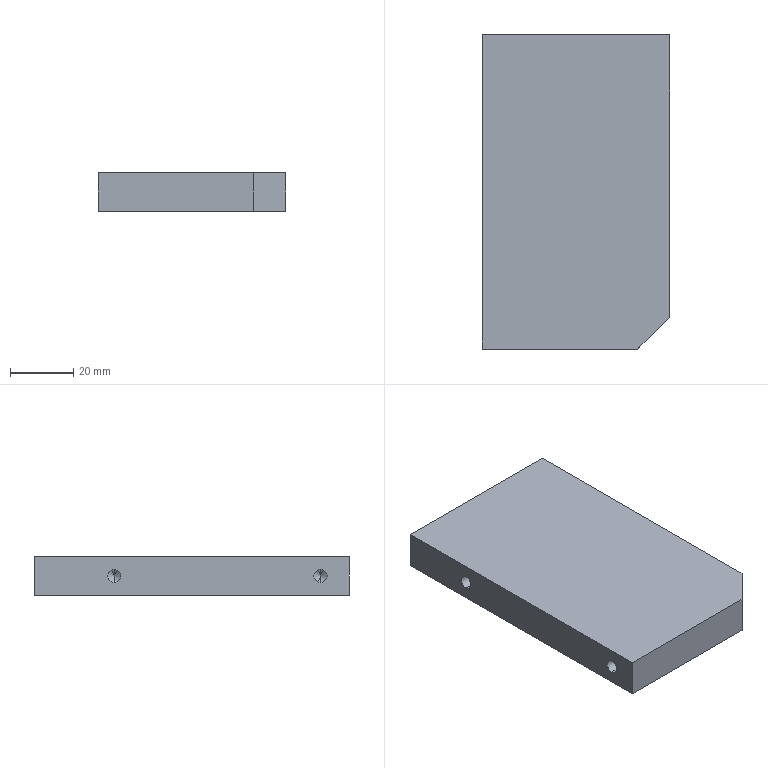Part | STEP file | 0245_202_Rib | 1 solid | 23 faces | box 59 x 99 x 12 mm | volume 68782 mm3 | cylinder 8 | cone 8 | plane 7 | commonest cylinder face diameters 4.2 x8
STEP:
#1=CARTESIAN_POINT('',(0.,0.,0.));
#2=DIRECTION('',(0.,0.,1.));
#3=DIRECTION('',(1.,0.,0.));
#4=AXIS2_PLACEMENT_3D('',#1,#2,#3);
#5=CARTESIAN_POINT('',(50.,-12.4,-3.9));
#6=VERTEX_POINT('',#5);
#7=CARTESIAN_POINT('',(50.,0.,-3.9));
#8=VERTEX_POINT('',#7);
#9=CARTESIAN_POINT('',(50.,0.,-3.9));
#10=DIRECTION('',(0.,1.,0.));
#11=VECTOR('',#10,1.);
#12=LINE('',#9,#11);
#13=CARTESIAN_POINT('',(50.,0.,-6.));
#14=DIRECTION('',(0.,1.,0.));
#15=DIRECTION('',(0.,0.,1.));
#16=AXIS2_PLACEMENT_3D('',#13,#14,#15);
#17=CYLINDRICAL_SURFACE('',#16,2.1);
#18=CARTESIAN_POINT('',(6.283,0.));
#19=DIRECTION('',(0.,1.));
#20=VECTOR('',#19,1.);
#21=LINE('',#18,#20);
#22=(GEOMETRIC_REPRESENTATION_CONTEXT(2)PARAMETRIC_REPRESENTATION_CONTEXT()REPRESENTATION_CONTEXT('',''));
#23=DEFINITIONAL_REPRESENTATION('',(#21),#22);
#24=PCURVE('',#17,#23);
#25=CARTESIAN_POINT('',(50.,0.,-6.));
#26=DIRECTION('',(0.,1.,0.));
#27=DIRECTION('',(0.,0.,1.));
#28=AXIS2_PLACEMENT_3D('',#25,#26,#27);
#29=CYLINDRICAL_SURFACE('',#28,2.1);
#30=CARTESIAN_POINT('',(0.,0.));
#31=DIRECTION('',(0.,1.));
#32=VECTOR('',#31,1.);
#33=LINE('',#30,#32);
#34=(GEOMETRIC_REPRESENTATION_CONTEXT(2)PARAMETRIC_REPRESENTATION_CONTEXT()REPRESENTATION_CONTEXT('',''));
#35=DEFINITIONAL_REPRESENTATION('',(#33),#34);
#36=PCURVE('',#29,#35);
#37=SURFACE_CURVE('',#12,(#24,#36),.PCURVE_S1.);
#38=EDGE_CURVE('',#6,#8,#37,.T.);
#39=ORIENTED_EDGE('',*,*,#38,.T.);
#40=CARTESIAN_POINT('',(50.,0.,-8.1));
#41=VERTEX_POINT('',#40);
#42=CARTESIAN_POINT('',(50.,0.,-6.));
#43=DIRECTION('',(0.,1.,0.));
#44=DIRECTION('',(0.,0.,1.));
#45=AXIS2_PLACEMENT_3D('',#42,#43,#44);
#46=CIRCLE('',#45,2.1);
#47=CARTESIAN_POINT('',(0.,0.));
#48=DIRECTION('',(1.,0.));
#49=VECTOR('',#48,1.);
#50=LINE('',#47,#49);
#51=(GEOMETRIC_REPRESENTATION_CONTEXT(2)PARAMETRIC_REPRESENTATION_CONTEXT()REPRESENTATION_CONTEXT('',''));
#52=DEFINITIONAL_REPRESENTATION('',(#50),#51);
#53=PCURVE('',#17,#52);
#54=CARTESIAN_POINT('',(0.,0.,-12.));
#55=DIRECTION('',(0.,1.,0.));
#56=DIRECTION('',(0.,0.,1.));
#57=AXIS2_PLACEMENT_3D('',#54,#55,#56);
#58=PLANE('',#57);
#59=CARTESIAN_POINT('',(6.,50.));
#60=DIRECTION('',(1.,0.));
#61=AXIS2_PLACEMENT_2D('',#59,#60);
#62=CIRCLE('',#61,2.1);
#63=(GEOMETRIC_REPRESENTATION_CONTEXT(2)PARAMETRIC_REPRESENTATION_CONTEXT()REPRESENTATION_CONTEXT('',''));
#64=DEFINITIONAL_REPRESENTATION('',(#62),#63);
#65=PCURVE('',#58,#64);
#66=SURFACE_CURVE('',#46,(#53,#65),.PCURVE_S1.);
#67=EDGE_CURVE('',#41,#8,#66,.T.);
#68=ORIENTED_EDGE('',*,*,#67,.F.);
#69=CARTESIAN_POINT('',(50.,-12.4,-8.1));
#70=VERTEX_POINT('',#69);
#71=CARTESIAN_POINT('',(50.,0.,-8.1));
#72=DIRECTION('',(0.,1.,0.));
#73=VECTOR('',#72,1.);
#74=LINE('',#71,#73);
#75=CARTESIAN_POINT('',(3.142,0.));
#76=DIRECTION('',(0.,1.));
#77=VECTOR('',#76,1.);
#78=LINE('',#75,#77);
#79=(GEOMETRIC_REPRESENTATION_CONTEXT(2)PARAMETRIC_REPRESENTATION_CONTEXT()REPRESENTATION_CONTEXT('',''));
#80=DEFINITIONAL_REPRESENTATION('',(#78),#79);
#81=PCURVE('',#17,#80);
#82=CARTESIAN_POINT('',(3.142,0.));
#83=DIRECTION('',(0.,1.));
#84=VECTOR('',#83,1.);
#85=LINE('',#82,#84);
#86=(GEOMETRIC_REPRESENTATION_CONTEXT(2)PARAMETRIC_REPRESENTATION_CONTEXT()REPRESENTATION_CONTEXT('',''));
#87=DEFINITIONAL_REPRESENTATION('',(#85),#86);
#88=PCURVE('',#29,#87);
#89=SURFACE_CURVE('',#74,(#81,#88),.PCURVE_S1.);
#90=EDGE_CURVE('',#70,#41,#89,.T.);
#91=ORIENTED_EDGE('',*,*,#90,.F.);
#92=CARTESIAN_POINT('',(50.,-12.4,-6.));
#93=DIRECTION('',(0.,1.,0.));
#94=DIRECTION('',(0.,0.,1.));
#95=AXIS2_PLACEMENT_3D('',#92,#93,#94);
#96=CIRCLE('',#95,2.1);
#97=CARTESIAN_POINT('',(0.,-12.4));
#98=DIRECTION('',(1.,0.));
#99=VECTOR('',#98,1.);
#100=LINE('',#97,#99);
#101=(GEOMETRIC_REPRESENTATION_CONTEXT(2)PARAMETRIC_REPRESENTATION_CONTEXT()REPRESENTATION_CONTEXT('',''));
#102=DEFINITIONAL_REPRESENTATION('',(#100),#101);
#103=PCURVE('',#17,#102);
#104=CARTESIAN_POINT('',(50.,-12.4,-6.));
#105=DIRECTION('',(0.,1.,0.));
#106=DIRECTION('',(0.,0.,1.));
#107=AXIS2_PLACEMENT_3D('',#104,#105,#106);
#108=CONICAL_SURFACE('',#107,2.1,1.03);
#109=CARTESIAN_POINT('',(0.,0.));
#110=DIRECTION('',(1.,0.));
#111=VECTOR('',#110,1.);
#112=LINE('',#109,#111);
#113=(GEOMETRIC_REPRESENTATION_CONTEXT(2)PARAMETRIC_REPRESENTATION_CONTEXT()REPRESENTATION_CONTEXT('',''));
#114=DEFINITIONAL_REPRESENTATION('',(#112),#113);
#115=PCURVE('',#108,#114);
#116=SURFACE_CURVE('',#96,(#103,#115),.PCURVE_S1.);
#117=EDGE_CURVE('',#70,#6,#116,.T.);
#118=ORIENTED_EDGE('',*,*,#117,.T.);
#119=EDGE_LOOP('',(#39,#68,#91,#118));
#120=FACE_BOUND('',#119,.F.);
#121=ADVANCED_FACE('',(#120),#17,.F.);
#122=ORIENTED_EDGE('',*,*,#117,.F.);
#123=CARTESIAN_POINT('',(50.,-13.662,-6.));
#124=VERTEX_POINT('',#123);
#125=CARTESIAN_POINT('',(50.,-12.4,-8.1));
#126=DIRECTION('',(0.,0.515,-0.8572));
#127=VECTOR('',#126,1.);
#128=LINE('',#125,#127);
#129=CARTESIAN_POINT('',(3.142,-1.262));
#130=CARTESIAN_POINT('',(3.142,-1.243));
#131=CARTESIAN_POINT('',(3.142,-1.204));
#132=CARTESIAN_POINT('',(3.142,-1.147));
#133=CARTESIAN_POINT('',(3.142,-1.09));
#134=CARTESIAN_POINT('',(3.142,-1.032));
#135=CARTESIAN_POINT('',(3.142,-0.975));
#136=CARTESIAN_POINT('',(3.142,-0.9177));
#137=CARTESIAN_POINT('',(3.142,-0.8603));
#138=CARTESIAN_POINT('',(3.142,-0.803));
#139=CARTESIAN_POINT('',(3.142,-0.7456));
#140=CARTESIAN_POINT('',(3.142,-0.6883));
#141=CARTESIAN_POINT('',(3.142,-0.6309));
#142=CARTESIAN_POINT('',(3.142,-0.5735));
#143=CARTESIAN_POINT('',(3.142,-0.5162));
#144=CARTESIAN_POINT('',(3.142,-0.4588));
#145=CARTESIAN_POINT('',(3.142,-0.4015));
#146=CARTESIAN_POINT('',(3.142,-0.3441));
#147=CARTESIAN_POINT('',(3.142,-0.2868));
#148=CARTESIAN_POINT('',(3.142,-0.2294));
#149=CARTESIAN_POINT('',(3.142,-0.1721));
#150=CARTESIAN_POINT('',(3.142,-0.1147));
#151=CARTESIAN_POINT('',(3.142,-0.05735));
#152=CARTESIAN_POINT('',(3.142,-0.01912));
#153=CARTESIAN_POINT('',(3.142,0.));
#154=B_SPLINE_CURVE_WITH_KNOTS('',3,(#129,#130,#131,#132,#133,#134,#135,#136,#137,#138,#139,#140,#141,#142,#143,#144,#145,#146,#147,#148,#149,#150,#151,#152,#153),.UNSPECIFIED.,.F.,.F.,(4,1,1,1,1,1,1,1,1,1,1,1,1,1,1,1,1,1,1,1,1,1,4),(-2.45,-2.339,-2.227,-2.116,-2.004,-1.893,-1.782,-1.67,-1.559,-1.448,-1.336,-1.225,-1.114,-1.002,-0.8909,-0.7795,-0.6682,-0.5568,-0.4454,-0.3341,-0.2227,-0.1114,0.),.UNSPECIFIED.);
#155=(GEOMETRIC_REPRESENTATION_CONTEXT(2)PARAMETRIC_REPRESENTATION_CONTEXT()REPRESENTATION_CONTEXT('',''));
#156=DEFINITIONAL_REPRESENTATION('',(#154),#155);
#157=PCURVE('',#108,#156);
#158=CARTESIAN_POINT('',(50.,-12.4,-6.));
#159=DIRECTION('',(0.,1.,0.));
#160=DIRECTION('',(0.,0.,1.));
#161=AXIS2_PLACEMENT_3D('',#158,#159,#160);
#162=CONICAL_SURFACE('',#161,2.1,1.03);
#163=CARTESIAN_POINT('',(3.142,-1.262));
#164=CARTESIAN_POINT('',(3.142,-1.243));
#165=CARTESIAN_POINT('',(3.142,-1.204));
#166=CARTESIAN_POINT('',(3.142,-1.147));
#167=CARTESIAN_POINT('',(3.142,-1.09));
#168=CARTESIAN_POINT('',(3.142,-1.032));
#169=CARTESIAN_POINT('',(3.142,-0.975));
#170=CARTESIAN_POINT('',(3.142,-0.9177));
#171=CARTESIAN_POINT('',(3.142,-0.8603));
#172=CARTESIAN_POINT('',(3.142,-0.803));
#173=CARTESIAN_POINT('',(3.142,-0.7456));
#174=CARTESIAN_POINT('',(3.142,-0.6883));
#175=CARTESIAN_POINT('',(3.142,-0.6309));
#176=CARTESIAN_POINT('',(3.142,-0.5735));
#177=CARTESIAN_POINT('',(3.142,-0.5162));
#178=CARTESIAN_POINT('',(3.142,-0.4588));
#179=CARTESIAN_POINT('',(3.142,-0.4015));
#180=CARTESIAN_POINT('',(3.142,-0.3441));
#181=CARTESIAN_POINT('',(3.142,-0.2868));
#182=CARTESIAN_POINT('',(3.142,-0.2294));
#183=CARTESIAN_POINT('',(3.142,-0.1721));
#184=CARTESIAN_POINT('',(3.142,-0.1147));
#185=CARTESIAN_POINT('',(3.142,-0.05735));
#186=CARTESIAN_POINT('',(3.142,-0.01912));
#187=CARTESIAN_POINT('',(3.142,0.));
#188=B_SPLINE_CURVE_WITH_KNOTS('',3,(#163,#164,#165,#166,#167,#168,#169,#170,#171,#172,#173,#174,#175,#176,#177,#178,#179,#180,#181,#182,#183,#184,#185,#186,#187),.UNSPECIFIED.,.F.,.F.,(4,1,1,1,1,1,1,1,1,1,1,1,1,1,1,1,1,1,1,1,1,1,4),(-2.45,-2.339,-2.227,-2.116,-2.004,-1.893,-1.782,-1.67,-1.559,-1.448,-1.336,-1.225,-1.114,-1.002,-0.8909,-0.7795,-0.6682,-0.5568,-0.4454,-0.3341,-0.2227,-0.1114,0.),.UNSPECIFIED.);
#189=(GEOMETRIC_REPRESENTATION_CONTEXT(2)PARAMETRIC_REPRESENTATION_CONTEXT()REPRESENTATION_CONTEXT('',''));
#190=DEFINITIONAL_REPRESENTATION('',(#188),#189);
#191=PCURVE('',#162,#190);
#192=SURFACE_CURVE('',#128,(#157,#191),.PCURVE_S1.);
#193=EDGE_CURVE('',#124,#70,#192,.T.);
#194=ORIENTED_EDGE('',*,*,#193,.F.);
#195=CARTESIAN_POINT('',(50.,-12.4,-3.9));
#196=DIRECTION('',(0.,0.515,0.8572));
#197=VECTOR('',#196,1.);
#198=LINE('',#195,#197);
#199=CARTESIAN_POINT('',(6.283,0.));
#200=DIRECTION('',(0.,1.));
#201=VECTOR('',#200,1.);
#202=LINE('',#199,#201);
#203=(GEOMETRIC_REPRESENTATION_CONTEXT(2)PARAMETRIC_REPRESENTATION_CONTEXT()REPRESENTATION_CONTEXT('',''));
#204=DEFINITIONAL_REPRESENTATION('',(#202),#203);
#205=PCURVE('',#108,#204);
#206=CARTESIAN_POINT('',(0.,0.));
#207=DIRECTION('',(0.,1.));
#208=VECTOR('',#207,1.);
#209=LINE('',#206,#208);
#210=(GEOMETRIC_REPRESENTATION_CONTEXT(2)PARAMETRIC_REPRESENTATION_CONTEXT()REPRESENTATION_CONTEXT('',''));
#211=DEFINITIONAL_REPRESENTATION('',(#209),#210);
#212=PCURVE('',#162,#211);
#213=SURFACE_CURVE('',#198,(#205,#212),.PCURVE_S1.);
#214=EDGE_CURVE('',#124,#6,#213,.T.);
#215=ORIENTED_EDGE('',*,*,#214,.T.);
#216=EDGE_LOOP('',(#122,#194,#215));
#217=FACE_BOUND('',#216,.F.);
#218=ADVANCED_FACE('',(#217),#108,.F.);
#219=CARTESIAN_POINT('',(20.,-12.4,-3.9));
#220=VERTEX_POINT('',#219);
#221=CARTESIAN_POINT('',(20.,0.,-3.9));
#222=VERTEX_POINT('',#221);
#223=CARTESIAN_POINT('',(20.,0.,-3.9));
#224=DIRECTION('',(0.,1.,0.));
#225=VECTOR('',#224,1.);
#226=LINE('',#223,#225);
#227=CARTESIAN_POINT('',(20.,0.,-6.));
#228=DIRECTION('',(0.,1.,0.));
#229=DIRECTION('',(0.,0.,1.));
#230=AXIS2_PLACEMENT_3D('',#227,#228,#229);
#231=CYLINDRICAL_SURFACE('',#230,2.1);
#232=CARTESIAN_POINT('',(6.283,0.));
#233=DIRECTION('',(0.,1.));
#234=VECTOR('',#233,1.);
#235=LINE('',#232,#234);
#236=(GEOMETRIC_REPRESENTATION_CONTEXT(2)PARAMETRIC_REPRESENTATION_CONTEXT()REPRESENTATION_CONTEXT('',''));
#237=DEFINITIONAL_REPRESENTATION('',(#235),#236);
#238=PCURVE('',#231,#237);
#239=CARTESIAN_POINT('',(20.,0.,-6.));
#240=DIRECTION('',(0.,1.,0.));
#241=DIRECTION('',(0.,0.,1.));
#242=AXIS2_PLACEMENT_3D('',#239,#240,#241);
#243=CYLINDRICAL_SURFACE('',#242,2.1);
#244=CARTESIAN_POINT('',(0.,0.));
#245=DIRECTION('',(0.,1.));
#246=VECTOR('',#245,1.);
#247=LINE('',#244,#246);
#248=(GEOMETRIC_REPRESENTATION_CONTEXT(2)PARAMETRIC_REPRESENTATION_CONTEXT()REPRESENTATION_CONTEXT('',''));
#249=DEFINITIONAL_REPRESENTATION('',(#247),#248);
#250=PCURVE('',#243,#249);
#251=SURFACE_CURVE('',#226,(#238,#250),.PCURVE_S1.);
#252=EDGE_CURVE('',#220,#222,#251,.T.);
#253=ORIENTED_EDGE('',*,*,#252,.T.);
#254=CARTESIAN_POINT('',(20.,0.,-8.1));
#255=VERTEX_POINT('',#254);
#256=CARTESIAN_POINT('',(20.,0.,-6.));
#257=DIRECTION('',(0.,1.,0.));
#258=DIRECTION('',(0.,0.,1.));
#259=AXIS2_PLACEMENT_3D('',#256,#257,#258);
#260=CIRCLE('',#259,2.1);
#261=CARTESIAN_POINT('',(0.,0.));
#262=DIRECTION('',(1.,0.));
#263=VECTOR('',#262,1.);
#264=LINE('',#261,#263);
#265=(GEOMETRIC_REPRESENTATION_CONTEXT(2)PARAMETRIC_REPRESENTATION_CONTEXT()REPRESENTATION_CONTEXT('',''));
#266=DEFINITIONAL_REPRESENTATION('',(#264),#265);
#267=PCURVE('',#231,#266);
#268=CARTESIAN_POINT('',(6.,20.));
#269=DIRECTION('',(1.,0.));
#270=AXIS2_PLACEMENT_2D('',#268,#269);
#271=CIRCLE('',#270,2.1);
#272=(GEOMETRIC_REPRESENTATION_CONTEXT(2)PARAMETRIC_REPRESENTATION_CONTEXT()REPRESENTATION_CONTEXT('',''));
#273=DEFINITIONAL_REPRESENTATION('',(#271),#272);
#274=PCURVE('',#58,#273);
#275=SURFACE_CURVE('',#260,(#267,#274),.PCURVE_S1.);
#276=EDGE_CURVE('',#255,#222,#275,.T.);
#277=ORIENTED_EDGE('',*,*,#276,.F.);
#278=CARTESIAN_POINT('',(20.,-12.4,-8.1));
#279=VERTEX_POINT('',#278);
#280=CARTESIAN_POINT('',(20.,0.,-8.1));
#281=DIRECTION('',(0.,1.,0.));
#282=VECTOR('',#281,1.);
#283=LINE('',#280,#282);
#284=CARTESIAN_POINT('',(3.142,0.));
#285=DIRECTION('',(0.,1.));
#286=VECTOR('',#285,1.);
#287=LINE('',#284,#286);
#288=(GEOMETRIC_REPRESENTATION_CONTEXT(2)PARAMETRIC_REPRESENTATION_CONTEXT()REPRESENTATION_CONTEXT('',''));
#289=DEFINITIONAL_REPRESENTATION('',(#287),#288);
#290=PCURVE('',#231,#289);
#291=CARTESIAN_POINT('',(3.142,0.));
#292=DIRECTION('',(0.,1.));
#293=VECTOR('',#292,1.);
#294=LINE('',#291,#293);
#295=(GEOMETRIC_REPRESENTATION_CONTEXT(2)PARAMETRIC_REPRESENTATION_CONTEXT()REPRESENTATION_CONTEXT('',''));
#296=DEFINITIONAL_REPRESENTATION('',(#294),#295);
#297=PCURVE('',#243,#296);
#298=SURFACE_CURVE('',#283,(#290,#297),.PCURVE_S1.);
#299=EDGE_CURVE('',#279,#255,#298,.T.);
#300=ORIENTED_EDGE('',*,*,#299,.F.);
#301=CARTESIAN_POINT('',(20.,-12.4,-6.));
#302=DIRECTION('',(0.,1.,0.));
#303=DIRECTION('',(0.,0.,1.));
#304=AXIS2_PLACEMENT_3D('',#301,#302,#303);
#305=CIRCLE('',#304,2.1);
#306=CARTESIAN_POINT('',(0.,-12.4));
#307=DIRECTION('',(1.,0.));
#308=VECTOR('',#307,1.);
#309=LINE('',#306,#308);
#310=(GEOMETRIC_REPRESENTATION_CONTEXT(2)PARAMETRIC_REPRESENTATION_CONTEXT()REPRESENTATION_CONTEXT('',''));
#311=DEFINITIONAL_REPRESENTATION('',(#309),#310);
#312=PCURVE('',#231,#311);
#313=CARTESIAN_POINT('',(20.,-12.4,-6.));
#314=DIRECTION('',(0.,1.,0.));
#315=DIRECTION('',(0.,0.,1.));
#316=AXIS2_PLACEMENT_3D('',#313,#314,#315);
#317=CONICAL_SURFACE('',#316,2.1,1.03);
#318=CARTESIAN_POINT('',(0.,0.));
#319=DIRECTION('',(1.,0.));
#320=VECTOR('',#319,1.);
#321=LINE('',#318,#320);
#322=(GEOMETRIC_REPRESENTATION_CONTEXT(2)PARAMETRIC_REPRESENTATION_CONTEXT()REPRESENTATION_CONTEXT('',''));
#323=DEFINITIONAL_REPRESENTATION('',(#321),#322);
#324=PCURVE('',#317,#323);
#325=SURFACE_CURVE('',#305,(#312,#324),.PCURVE_S1.);
#326=EDGE_CURVE('',#279,#220,#325,.T.);
#327=ORIENTED_EDGE('',*,*,#326,.T.);
#328=EDGE_LOOP('',(#253,#277,#300,#327));
#329=FACE_BOUND('',#328,.F.);
#330=ADVANCED_FACE('',(#329),#231,.F.);
#331=ORIENTED_EDGE('',*,*,#326,.F.);
#332=CARTESIAN_POINT('',(20.,-13.662,-6.));
#333=VERTEX_POINT('',#332);
#334=CARTESIAN_POINT('',(20.,-12.4,-8.1));
#335=DIRECTION('',(0.,0.515,-0.8572));
#336=VECTOR('',#335,1.);
#337=LINE('',#334,#336);
#338=CARTESIAN_POINT('',(3.142,0.));
#339=DIRECTION('',(0.,1.));
#340=VECTOR('',#339,1.);
#341=LINE('',#338,#340);
#342=(GEOMETRIC_REPRESENTATION_CONTEXT(2)PARAMETRIC_REPRESENTATION_CONTEXT()REPRESENTATION_CONTEXT('',''));
#343=DEFINITIONAL_REPRESENTATION('',(#341),#342);
#344=PCURVE('',#317,#343);
#345=CARTESIAN_POINT('',(20.,-12.4,-6.));
#346=DIRECTION('',(0.,1.,0.));
#347=DIRECTION('',(0.,0.,1.));
#348=AXIS2_PLACEMENT_3D('',#345,#346,#347);
#349=CONICAL_SURFACE('',#348,2.1,1.03);
#350=CARTESIAN_POINT('',(3.142,0.));
#351=DIRECTION('',(0.,1.));
#352=VECTOR('',#351,1.);
#353=LINE('',#350,#352);
#354=(GEOMETRIC_REPRESENTATION_CONTEXT(2)PARAMETRIC_REPRESENTATION_CONTEXT()REPRESENTATION_CONTEXT('',''));
#355=DEFINITIONAL_REPRESENTATION('',(#353),#354);
#356=PCURVE('',#349,#355);
#357=SURFACE_CURVE('',#337,(#344,#356),.PCURVE_S1.);
#358=EDGE_CURVE('',#333,#279,#357,.T.);
#359=ORIENTED_EDGE('',*,*,#358,.F.);
#360=CARTESIAN_POINT('',(20.,-12.4,-3.9));
#361=DIRECTION('',(0.,0.515,0.8572));
#362=VECTOR('',#361,1.);
#363=LINE('',#360,#362);
#364=CARTESIAN_POINT('',(6.283,0.));
#365=DIRECTION('',(0.,1.));
#366=VECTOR('',#365,1.);
#367=LINE('',#364,#366);
#368=(GEOMETRIC_REPRESENTATION_CONTEXT(2)PARAMETRIC_REPRESENTATION_CONTEXT()REPRESENTATION_CONTEXT('',''));
#369=DEFINITIONAL_REPRESENTATION('',(#367),#368);
#370=PCURVE('',#317,#369);
#371=CARTESIAN_POINT('',(0.,0.));
#372=DIRECTION('',(0.,1.));
#373=VECTOR('',#372,1.);
#374=LINE('',#371,#373);
#375=(GEOMETRIC_REPRESENTATION_CONTEXT(2)PARAMETRIC_REPRESENTATION_CONTEXT()REPRESENTATION_CONTEXT('',''));
#376=DEFINITIONAL_REPRESENTATION('',(#374),#375);
#377=PCURVE('',#349,#376);
#378=SURFACE_CURVE('',#363,(#370,#377),.PCURVE_S1.);
#379=EDGE_CURVE('',#333,#220,#378,.T.);
#380=ORIENTED_EDGE('',*,*,#379,.T.);
#381=EDGE_LOOP('',(#331,#359,#380));
#382=FACE_BOUND('',#381,.F.);
#383=ADVANCED_FACE('',(#382),#317,.F.);
#384=CARTESIAN_POINT('',(12.4,-25.,-3.9));
#385=VERTEX_POINT('',#384);
#386=CARTESIAN_POINT('',(0.,-25.,-3.9));
#387=VERTEX_POINT('',#386);
#388=CARTESIAN_POINT('',(0.,-25.,-3.9));
#389=DIRECTION('',(-1.,0.,0.));
#390=VECTOR('',#389,1.);
#391=LINE('',#388,#390);
#392=CARTESIAN_POINT('',(0.,-25.,-6.));
#393=DIRECTION('',(-1.,0.,0.));
#394=DIRECTION('',(0.,0.,1.));
#395=AXIS2_PLACEMENT_3D('',#392,#393,#394);
#396=CYLINDRICAL_SURFACE('',#395,2.1);
#397=CARTESIAN_POINT('',(6.283,0.));
#398=DIRECTION('',(0.,1.));
#399=VECTOR('',#398,1.);
#400=LINE('',#397,#399);
#401=(GEOMETRIC_REPRESENTATION_CONTEXT(2)PARAMETRIC_REPRESENTATION_CONTEXT()REPRESENTATION_CONTEXT('',''));
#402=DEFINITIONAL_REPRESENTATION('',(#400),#401);
#403=PCURVE('',#396,#402);
#404=CARTESIAN_POINT('',(0.,-25.,-6.));
#405=DIRECTION('',(-1.,0.,0.));
#406=DIRECTION('',(0.,0.,1.));
#407=AXIS2_PLACEMENT_3D('',#404,#405,#406);
#408=CYLINDRICAL_SURFACE('',#407,2.1);
#409=CARTESIAN_POINT('',(0.,0.));
#410=DIRECTION('',(0.,1.));
#411=VECTOR('',#410,1.);
#412=LINE('',#409,#411);
#413=(GEOMETRIC_REPRESENTATION_CONTEXT(2)PARAMETRIC_REPRESENTATION_CONTEXT()REPRESENTATION_CONTEXT('',''));
#414=DEFINITIONAL_REPRESENTATION('',(#412),#413);
#415=PCURVE('',#408,#414);
#416=SURFACE_CURVE('',#391,(#403,#415),.PCURVE_S1.);
#417=EDGE_CURVE('',#385,#387,#416,.T.);
#418=ORIENTED_EDGE('',*,*,#417,.T.);
#419=CARTESIAN_POINT('',(0.,-25.,-8.1));
#420=VERTEX_POINT('',#419);
#421=CARTESIAN_POINT('',(0.,-25.,-6.));
#422=DIRECTION('',(-1.,0.,0.));
#423=DIRECTION('',(0.,0.,1.));
#424=AXIS2_PLACEMENT_3D('',#421,#422,#423);
#425=CIRCLE('',#424,2.1);
#426=CARTESIAN_POINT('',(0.,0.));
#427=DIRECTION('',(1.,0.));
#428=VECTOR('',#427,1.);
#429=LINE('',#426,#428);
#430=(GEOMETRIC_REPRESENTATION_CONTEXT(2)PARAMETRIC_REPRESENTATION_CONTEXT()REPRESENTATION_CONTEXT('',''));
#431=DEFINITIONAL_REPRESENTATION('',(#429),#430);
#432=PCURVE('',#396,#431);
#433=CARTESIAN_POINT('',(0.,-99.,-12.));
#434=DIRECTION('',(-1.,0.,0.));
#435=DIRECTION('',(0.,0.,1.));
#436=AXIS2_PLACEMENT_3D('',#433,#434,#435);
#437=PLANE('',#436);
#438=CARTESIAN_POINT('',(6.,74.));
#439=DIRECTION('',(1.,0.));
#440=AXIS2_PLACEMENT_2D('',#438,#439);
#441=CIRCLE('',#440,2.1);
#442=(GEOMETRIC_REPRESENTATION_CONTEXT(2)PARAMETRIC_REPRESENTATION_CONTEXT()REPRESENTATION_CONTEXT('',''));
#443=DEFINITIONAL_REPRESENTATION('',(#441),#442);
#444=PCURVE('',#437,#443);
#445=SURFACE_CURVE('',#425,(#432,#444),.PCURVE_S1.);
#446=EDGE_CURVE('',#420,#387,#445,.T.);
#447=ORIENTED_EDGE('',*,*,#446,.F.);
#448=CARTESIAN_POINT('',(12.4,-25.,-8.1));
#449=VERTEX_POINT('',#448);
#450=CARTESIAN_POINT('',(0.,-25.,-8.1));
#451=DIRECTION('',(-1.,0.,0.));
#452=VECTOR('',#451,1.);
#453=LINE('',#450,#452);
#454=CARTESIAN_POINT('',(3.142,0.));
#455=DIRECTION('',(0.,1.));
#456=VECTOR('',#455,1.);
#457=LINE('',#454,#456);
#458=(GEOMETRIC_REPRESENTATION_CONTEXT(2)PARAMETRIC_REPRESENTATION_CONTEXT()REPRESENTATION_CONTEXT('',''));
#459=DEFINITIONAL_REPRESENTATION('',(#457),#458);
#460=PCURVE('',#396,#459);
#461=CARTESIAN_POINT('',(3.142,0.));
#462=DIRECTION('',(0.,1.));
#463=VECTOR('',#462,1.);
#464=LINE('',#461,#463);
#465=(GEOMETRIC_REPRESENTATION_CONTEXT(2)PARAMETRIC_REPRESENTATION_CONTEXT()REPRESENTATION_CONTEXT('',''));
#466=DEFINITIONAL_REPRESENTATION('',(#464),#465);
#467=PCURVE('',#408,#466);
#468=SURFACE_CURVE('',#453,(#460,#467),.PCURVE_S1.);
#469=EDGE_CURVE('',#449,#420,#468,.T.);
#470=ORIENTED_EDGE('',*,*,#469,.F.);
#471=CARTESIAN_POINT('',(12.4,-25.,-6.));
#472=DIRECTION('',(-1.,0.,0.));
#473=DIRECTION('',(0.,0.,1.));
#474=AXIS2_PLACEMENT_3D('',#471,#472,#473);
#475=CIRCLE('',#474,2.1);
#476=CARTESIAN_POINT('',(0.,-12.4));
#477=DIRECTION('',(1.,0.));
#478=VECTOR('',#477,1.);
#479=LINE('',#476,#478);
#480=(GEOMETRIC_REPRESENTATION_CONTEXT(2)PARAMETRIC_REPRESENTATION_CONTEXT()REPRESENTATION_CONTEXT('',''));
#481=DEFINITIONAL_REPRESENTATION('',(#479),#480);
#482=PCURVE('',#396,#481);
#483=CARTESIAN_POINT('',(12.4,-25.,-6.));
#484=DIRECTION('',(-1.,0.,0.));
#485=DIRECTION('',(0.,0.,1.));
#486=AXIS2_PLACEMENT_3D('',#483,#484,#485);
#487=CONICAL_SURFACE('',#486,2.1,1.03);
#488=CARTESIAN_POINT('',(0.,0.));
#489=DIRECTION('',(1.,0.));
#490=VECTOR('',#489,1.);
#491=LINE('',#488,#490);
#492=(GEOMETRIC_REPRESENTATION_CONTEXT(2)PARAMETRIC_REPRESENTATION_CONTEXT()REPRESENTATION_CONTEXT('',''));
#493=DEFINITIONAL_REPRESENTATION('',(#491),#492);
#494=PCURVE('',#487,#493);
#495=SURFACE_CURVE('',#475,(#482,#494),.PCURVE_S1.);
#496=EDGE_CURVE('',#449,#385,#495,.T.);
#497=ORIENTED_EDGE('',*,*,#496,.T.);
#498=EDGE_LOOP('',(#418,#447,#470,#497));
#499=FACE_BOUND('',#498,.F.);
#500=ADVANCED_FACE('',(#499),#396,.F.);
#501=ORIENTED_EDGE('',*,*,#496,.F.);
#502=CARTESIAN_POINT('',(13.662,-25.,-6.));
#503=VERTEX_POINT('',#502);
#504=CARTESIAN_POINT('',(12.4,-25.,-8.1));
#505=DIRECTION('',(-0.515,0.,-0.8572));
#506=VECTOR('',#505,1.);
#507=LINE('',#504,#506);
#508=CARTESIAN_POINT('',(3.142,0.));
#509=DIRECTION('',(0.,1.));
#510=VECTOR('',#509,1.);
#511=LINE('',#508,#510);
#512=(GEOMETRIC_REPRESENTATION_CONTEXT(2)PARAMETRIC_REPRESENTATION_CONTEXT()REPRESENTATION_CONTEXT('',''));
#513=DEFINITIONAL_REPRESENTATION('',(#511),#512);
#514=PCURVE('',#487,#513);
#515=CARTESIAN_POINT('',(12.4,-25.,-6.));
#516=DIRECTION('',(-1.,0.,0.));
#517=DIRECTION('',(0.,0.,1.));
#518=AXIS2_PLACEMENT_3D('',#515,#516,#517);
#519=CONICAL_SURFACE('',#518,2.1,1.03);
#520=CARTESIAN_POINT('',(3.142,0.));
#521=DIRECTION('',(0.,1.));
#522=VECTOR('',#521,1.);
#523=LINE('',#520,#522);
#524=(GEOMETRIC_REPRESENTATION_CONTEXT(2)PARAMETRIC_REPRESENTATION_CONTEXT()REPRESENTATION_CONTEXT('',''));
#525=DEFINITIONAL_REPRESENTATION('',(#523),#524);
#526=PCURVE('',#519,#525);
#527=SURFACE_CURVE('',#507,(#514,#526),.PCURVE_S1.);
#528=EDGE_CURVE('',#503,#449,#527,.T.);
#529=ORIENTED_EDGE('',*,*,#528,.F.);
#530=CARTESIAN_POINT('',(12.4,-25.,-3.9));
#531=DIRECTION('',(-0.515,0.,0.8572));
#532=VECTOR('',#531,1.);
#533=LINE('',#530,#532);
#534=CARTESIAN_POINT('',(6.283,0.));
#535=DIRECTION('',(0.,1.));
#536=VECTOR('',#535,1.);
#537=LINE('',#534,#536);
#538=(GEOMETRIC_REPRESENTATION_CONTEXT(2)PARAMETRIC_REPRESENTATION_CONTEXT()REPRESENTATION_CONTEXT('',''));
#539=DEFINITIONAL_REPRESENTATION('',(#537),#538);
#540=PCURVE('',#487,#539);
#541=CARTESIAN_POINT('',(0.,0.));
#542=DIRECTION('',(0.,1.));
#543=VECTOR('',#542,1.);
#544=LINE('',#541,#543);
#545=(GEOMETRIC_REPRESENTATION_CONTEXT(2)PARAMETRIC_REPRESENTATION_CONTEXT()REPRESENTATION_CONTEXT('',''));
#546=DEFINITIONAL_REPRESENTATION('',(#544),#545);
#547=PCURVE('',#519,#546);
#548=SURFACE_CURVE('',#533,(#540,#547),.PCURVE_S1.);
#549=EDGE_CURVE('',#503,#385,#548,.T.);
#550=ORIENTED_EDGE('',*,*,#549,.T.);
#551=EDGE_LOOP('',(#501,#529,#550));
#552=FACE_BOUND('',#551,.F.);
#553=ADVANCED_FACE('',(#552),#487,.F.);
#554=CARTESIAN_POINT('',(12.4,-90.,-3.9));
#555=VERTEX_POINT('',#554);
#556=CARTESIAN_POINT('',(0.,-90.,-3.9));
#557=VERTEX_POINT('',#556);
#558=CARTESIAN_POINT('',(0.,-90.,-3.9));
#559=DIRECTION('',(-1.,0.,0.));
#560=VECTOR('',#559,1.);
#561=LINE('',#558,#560);
#562=CARTESIAN_POINT('',(0.,-90.,-6.));
#563=DIRECTION('',(-1.,0.,0.));
#564=DIRECTION('',(0.,0.,1.));
#565=AXIS2_PLACEMENT_3D('',#562,#563,#564);
#566=CYLINDRICAL_SURFACE('',#565,2.1);
#567=CARTESIAN_POINT('',(6.283,0.));
#568=DIRECTION('',(0.,1.));
#569=VECTOR('',#568,1.);
#570=LINE('',#567,#569);
#571=(GEOMETRIC_REPRESENTATION_CONTEXT(2)PARAMETRIC_REPRESENTATION_CONTEXT()REPRESENTATION_CONTEXT('',''));
#572=DEFINITIONAL_REPRESENTATION('',(#570),#571);
#573=PCURVE('',#566,#572);
#574=CARTESIAN_POINT('',(0.,-90.,-6.));
#575=DIRECTION('',(-1.,0.,0.));
#576=DIRECTION('',(0.,0.,1.));
#577=AXIS2_PLACEMENT_3D('',#574,#575,#576);
#578=CYLINDRICAL_SURFACE('',#577,2.1);
#579=CARTESIAN_POINT('',(0.,0.));
#580=DIRECTION('',(0.,1.));
#581=VECTOR('',#580,1.);
#582=LINE('',#579,#581);
#583=(GEOMETRIC_REPRESENTATION_CONTEXT(2)PARAMETRIC_REPRESENTATION_CONTEXT()REPRESENTATION_CONTEXT('',''));
#584=DEFINITIONAL_REPRESENTATION('',(#582),#583);
#585=PCURVE('',#578,#584);
#586=SURFACE_CURVE('',#561,(#573,#585),.PCURVE_S1.);
#587=EDGE_CURVE('',#555,#557,#586,.T.);
#588=ORIENTED_EDGE('',*,*,#587,.T.);
#589=CARTESIAN_POINT('',(0.,-90.,-8.1));
#590=VERTEX_POINT('',#589);
#591=CARTESIAN_POINT('',(0.,-90.,-6.));
#592=DIRECTION('',(-1.,0.,0.));
#593=DIRECTION('',(0.,0.,1.));
#594=AXIS2_PLACEMENT_3D('',#591,#592,#593);
#595=CIRCLE('',#594,2.1);
#596=CARTESIAN_POINT('',(0.,0.));
#597=DIRECTION('',(1.,0.));
#598=VECTOR('',#597,1.);
#599=LINE('',#596,#598);
#600=(GEOMETRIC_REPRESENTATION_CONTEXT(2)PARAMETRIC_REPRESENTATION_CONTEXT()REPRESENTATION_CONTEXT('',''));
#601=DEFINITIONAL_REPRESENTATION('',(#599),#600);
#602=PCURVE('',#566,#601);
#603=CARTESIAN_POINT('',(6.,9.));
#604=DIRECTION('',(1.,0.));
#605=AXIS2_PLACEMENT_2D('',#603,#604);
#606=CIRCLE('',#605,2.1);
#607=(GEOMETRIC_REPRESENTATION_CONTEXT(2)PARAMETRIC_REPRESENTATION_CONTEXT()REPRESENTATION_CONTEXT('',''));
#608=DEFINITIONAL_REPRESENTATION('',(#606),#607);
#609=PCURVE('',#437,#608);
#610=SURFACE_CURVE('',#595,(#602,#609),.PCURVE_S1.);
#611=EDGE_CURVE('',#590,#557,#610,.T.);
#612=ORIENTED_EDGE('',*,*,#611,.F.);
#613=CARTESIAN_POINT('',(12.4,-90.,-8.1));
#614=VERTEX_POINT('',#613);
#615=CARTESIAN_POINT('',(0.,-90.,-8.1));
#616=DIRECTION('',(-1.,0.,0.));
#617=VECTOR('',#616,1.);
#618=LINE('',#615,#617);
#619=CARTESIAN_POINT('',(3.142,0.));
#620=DIRECTION('',(0.,1.));
#621=VECTOR('',#620,1.);
#622=LINE('',#619,#621);
#623=(GEOMETRIC_REPRESENTATION_CONTEXT(2)PARAMETRIC_REPRESENTATION_CONTEXT()REPRESENTATION_CONTEXT('',''));
#624=DEFINITIONAL_REPRESENTATION('',(#622),#623);
#625=PCURVE('',#566,#624);
#626=CARTESIAN_POINT('',(3.142,0.));
#627=DIRECTION('',(0.,1.));
#628=VECTOR('',#627,1.);
#629=LINE('',#626,#628);
#630=(GEOMETRIC_REPRESENTATION_CONTEXT(2)PARAMETRIC_REPRESENTATION_CONTEXT()REPRESENTATION_CONTEXT('',''));
#631=DEFINITIONAL_REPRESENTATION('',(#629),#630);
#632=PCURVE('',#578,#631);
#633=SURFACE_CURVE('',#618,(#625,#632),.PCURVE_S1.);
#634=EDGE_CURVE('',#614,#590,#633,.T.);
#635=ORIENTED_EDGE('',*,*,#634,.F.);
#636=CARTESIAN_POINT('',(12.4,-90.,-6.));
#637=DIRECTION('',(-1.,0.,0.));
#638=DIRECTION('',(0.,0.,1.));
#639=AXIS2_PLACEMENT_3D('',#636,#637,#638);
#640=CIRCLE('',#639,2.1);
#641=CARTESIAN_POINT('',(0.,-12.4));
#642=DIRECTION('',(1.,0.));
#643=VECTOR('',#642,1.);
#644=LINE('',#641,#643);
#645=(GEOMETRIC_REPRESENTATION_CONTEXT(2)PARAMETRIC_REPRESENTATION_CONTEXT()REPRESENTATION_CONTEXT('',''));
#646=DEFINITIONAL_REPRESENTATION('',(#644),#645);
#647=PCURVE('',#566,#646);
#648=CARTESIAN_POINT('',(12.4,-90.,-6.));
#649=DIRECTION('',(-1.,0.,0.));
#650=DIRECTION('',(0.,0.,1.));
#651=AXIS2_PLACEMENT_3D('',#648,#649,#650);
#652=CONICAL_SURFACE('',#651,2.1,1.03);
#653=CARTESIAN_POINT('',(0.,0.));
#654=DIRECTION('',(1.,0.));
#655=VECTOR('',#654,1.);
#656=LINE('',#653,#655);
#657=(GEOMETRIC_REPRESENTATION_CONTEXT(2)PARAMETRIC_REPRESENTATION_CONTEXT()REPRESENTATION_CONTEXT('',''));
#658=DEFINITIONAL_REPRESENTATION('',(#656),#657);
#659=PCURVE('',#652,#658);
#660=SURFACE_CURVE('',#640,(#647,#659),.PCURVE_S1.);
#661=EDGE_CURVE('',#614,#555,#660,.T.);
#662=ORIENTED_EDGE('',*,*,#661,.T.);
#663=EDGE_LOOP('',(#588,#612,#635,#662));
#664=FACE_BOUND('',#663,.F.);
#665=ADVANCED_FACE('',(#664),#566,.F.);
#666=ORIENTED_EDGE('',*,*,#661,.F.);
#667=CARTESIAN_POINT('',(13.662,-90.,-6.));
#668=VERTEX_POINT('',#667);
#669=CARTESIAN_POINT('',(12.4,-90.,-8.1));
#670=DIRECTION('',(-0.515,0.,-0.8572));
#671=VECTOR('',#670,1.);
#672=LINE('',#669,#671);
#673=CARTESIAN_POINT('',(3.142,-1.262));
#674=CARTESIAN_POINT('',(3.142,-1.243));
#675=CARTESIAN_POINT('',(3.142,-1.204));
#676=CARTESIAN_POINT('',(3.142,-1.147));
#677=CARTESIAN_POINT('',(3.142,-1.09));
#678=CARTESIAN_POINT('',(3.142,-1.032));
#679=CARTESIAN_POINT('',(3.142,-0.975));
#680=CARTESIAN_POINT('',(3.142,-0.9177));
#681=CARTESIAN_POINT('',(3.142,-0.8603));
#682=CARTESIAN_POINT('',(3.142,-0.803));
#683=CARTESIAN_POINT('',(3.142,-0.7456));
#684=CARTESIAN_POINT('',(3.142,-0.6883));
#685=CARTESIAN_POINT('',(3.142,-0.6309));
#686=CARTESIAN_POINT('',(3.142,-0.5735));
#687=CARTESIAN_POINT('',(3.142,-0.5162));
#688=CARTESIAN_POINT('',(3.142,-0.4588));
#689=CARTESIAN_POINT('',(3.142,-0.4015));
#690=CARTESIAN_POINT('',(3.142,-0.3441));
#691=CARTESIAN_POINT('',(3.142,-0.2868));
#692=CARTESIAN_POINT('',(3.142,-0.2294));
#693=CARTESIAN_POINT('',(3.142,-0.1721));
#694=CARTESIAN_POINT('',(3.142,-0.1147));
#695=CARTESIAN_POINT('',(3.142,-0.05735));
#696=CARTESIAN_POINT('',(3.142,-0.01912));
#697=CARTESIAN_POINT('',(3.142,0.));
#698=B_SPLINE_CURVE_WITH_KNOTS('',3,(#673,#674,#675,#676,#677,#678,#679,#680,#681,#682,#683,#684,#685,#686,#687,#688,#689,#690,#691,#692,#693,#694,#695,#696,#697),.UNSPECIFIED.,.F.,.F.,(4,1,1,1,1,1,1,1,1,1,1,1,1,1,1,1,1,1,1,1,1,1,4),(-2.45,-2.339,-2.227,-2.116,-2.004,-1.893,-1.782,-1.67,-1.559,-1.448,-1.336,-1.225,-1.114,-1.002,-0.8909,-0.7795,-0.6682,-0.5568,-0.4454,-0.3341,-0.2227,-0.1114,0.),.UNSPECIFIED.);
#699=(GEOMETRIC_REPRESENTATION_CONTEXT(2)PARAMETRIC_REPRESENTATION_CONTEXT()REPRESENTATION_CONTEXT('',''));
#700=DEFINITIONAL_REPRESENTATION('',(#698),#699);
#701=PCURVE('',#652,#700);
#702=CARTESIAN_POINT('',(12.4,-90.,-6.));
#703=DIRECTION('',(-1.,0.,0.));
#704=DIRECTION('',(0.,0.,1.));
#705=AXIS2_PLACEMENT_3D('',#702,#703,#704);
#706=CONICAL_SURFACE('',#705,2.1,1.03);
#707=CARTESIAN_POINT('',(3.142,-1.262));
#708=CARTESIAN_POINT('',(3.142,-1.243));
#709=CARTESIAN_POINT('',(3.142,-1.204));
#710=CARTESIAN_POINT('',(3.142,-1.147));
#711=CARTESIAN_POINT('',(3.142,-1.09));
#712=CARTESIAN_POINT('',(3.142,-1.032));
#713=CARTESIAN_POINT('',(3.142,-0.975));
#714=CARTESIAN_POINT('',(3.142,-0.9177));
#715=CARTESIAN_POINT('',(3.142,-0.8603));
#716=CARTESIAN_POINT('',(3.142,-0.803));
#717=CARTESIAN_POINT('',(3.142,-0.7456));
#718=CARTESIAN_POINT('',(3.142,-0.6883));
#719=CARTESIAN_POINT('',(3.142,-0.6309));
#720=CARTESIAN_POINT('',(3.142,-0.5735));
#721=CARTESIAN_POINT('',(3.142,-0.5162));
#722=CARTESIAN_POINT('',(3.142,-0.4588));
#723=CARTESIAN_POINT('',(3.142,-0.4015));
#724=CARTESIAN_POINT('',(3.142,-0.3441));
#725=CARTESIAN_POINT('',(3.142,-0.2868));
#726=CARTESIAN_POINT('',(3.142,-0.2294));
#727=CARTESIAN_POINT('',(3.142,-0.1721));
#728=CARTESIAN_POINT('',(3.142,-0.1147));
#729=CARTESIAN_POINT('',(3.142,-0.05735));
#730=CARTESIAN_POINT('',(3.142,-0.01912));
#731=CARTESIAN_POINT('',(3.142,0.));
#732=B_SPLINE_CURVE_WITH_KNOTS('',3,(#707,#708,#709,#710,#711,#712,#713,#714,#715,#716,#717,#718,#719,#720,#721,#722,#723,#724,#725,#726,#727,#728,#729,#730,#731),.UNSPECIFIED.,.F.,.F.,(4,1,1,1,1,1,1,1,1,1,1,1,1,1,1,1,1,1,1,1,1,1,4),(-2.45,-2.339,-2.227,-2.116,-2.004,-1.893,-1.782,-1.67,-1.559,-1.448,-1.336,-1.225,-1.114,-1.002,-0.8909,-0.7795,-0.6682,-0.5568,-0.4454,-0.3341,-0.2227,-0.1114,0.),.UNSPECIFIED.);
#733=(GEOMETRIC_REPRESENTATION_CONTEXT(2)PARAMETRIC_REPRESENTATION_CONTEXT()REPRESENTATION_CONTEXT('',''));
#734=DEFINITIONAL_REPRESENTATION('',(#732),#733);
#735=PCURVE('',#706,#734);
#736=SURFACE_CURVE('',#672,(#701,#735),.PCURVE_S1.);
#737=EDGE_CURVE('',#668,#614,#736,.T.);
#738=ORIENTED_EDGE('',*,*,#737,.F.);
#739=CARTESIAN_POINT('',(12.4,-90.,-3.9));
#740=DIRECTION('',(-0.515,0.,0.8572));
#741=VECTOR('',#740,1.);
#742=LINE('',#739,#741);
#743=CARTESIAN_POINT('',(6.283,0.));
#744=DIRECTION('',(0.,1.));
#745=VECTOR('',#744,1.);
#746=LINE('',#743,#745);
#747=(GEOMETRIC_REPRESENTATION_CONTEXT(2)PARAMETRIC_REPRESENTATION_CONTEXT()REPRESENTATION_CONTEXT('',''));
#748=DEFINITIONAL_REPRESENTATION('',(#746),#747);
#749=PCURVE('',#652,#748);
#750=CARTESIAN_POINT('',(0.,0.));
#751=DIRECTION('',(0.,1.));
#752=VECTOR('',#751,1.);
#753=LINE('',#750,#752);
#754=(GEOMETRIC_REPRESENTATION_CONTEXT(2)PARAMETRIC_REPRESENTATION_CONTEXT()REPRESENTATION_CONTEXT('',''));
#755=DEFINITIONAL_REPRESENTATION('',(#753),#754);
#756=PCURVE('',#706,#755);
#757=SURFACE_CURVE('',#742,(#749,#756),.PCURVE_S1.);
#758=EDGE_CURVE('',#668,#555,#757,.T.);
#759=ORIENTED_EDGE('',*,*,#758,.T.);
#760=EDGE_LOOP('',(#666,#738,#759));
#761=FACE_BOUND('',#760,.F.);
#762=ADVANCED_FACE('',(#761),#652,.F.);
#763=CARTESIAN_POINT('',(0.,-25.,-6.));
#764=DIRECTION('',(-1.,0.,0.));
#765=DIRECTION('',(0.,0.,1.));
#766=AXIS2_PLACEMENT_3D('',#763,#764,#765);
#767=CIRCLE('',#766,2.1);
#768=CARTESIAN_POINT('',(6.,74.));
#769=DIRECTION('',(1.,0.));
#770=AXIS2_PLACEMENT_2D('',#768,#769);
#771=CIRCLE('',#770,2.1);
#772=(GEOMETRIC_REPRESENTATION_CONTEXT(2)PARAMETRIC_REPRESENTATION_CONTEXT()REPRESENTATION_CONTEXT('',''));
#773=DEFINITIONAL_REPRESENTATION('',(#771),#772);
#774=PCURVE('',#437,#773);
#775=CARTESIAN_POINT('',(0.,0.));
#776=DIRECTION('',(1.,0.));
#777=VECTOR('',#776,1.);
#778=LINE('',#775,#777);
#779=(GEOMETRIC_REPRESENTATION_CONTEXT(2)PARAMETRIC_REPRESENTATION_CONTEXT()REPRESENTATION_CONTEXT('',''));
#780=DEFINITIONAL_REPRESENTATION('',(#778),#779);
#781=PCURVE('',#408,#780);
#782=SURFACE_CURVE('',#767,(#774,#781),.PCURVE_S1.);
#783=EDGE_CURVE('',#387,#420,#782,.T.);
#784=ORIENTED_EDGE('',*,*,#783,.F.);
#785=ORIENTED_EDGE('',*,*,#446,.F.);
#786=EDGE_LOOP('',(#784,#785));
#787=FACE_BOUND('',#786,.T.);
#788=CARTESIAN_POINT('',(0.,-90.,-6.));
#789=DIRECTION('',(-1.,0.,0.));
#790=DIRECTION('',(0.,0.,1.));
#791=AXIS2_PLACEMENT_3D('',#788,#789,#790);
#792=CIRCLE('',#791,2.1);
#793=CARTESIAN_POINT('',(6.,9.));
#794=DIRECTION('',(1.,0.));
#795=AXIS2_PLACEMENT_2D('',#793,#794);
#796=CIRCLE('',#795,2.1);
#797=(GEOMETRIC_REPRESENTATION_CONTEXT(2)PARAMETRIC_REPRESENTATION_CONTEXT()REPRESENTATION_CONTEXT('',''));
#798=DEFINITIONAL_REPRESENTATION('',(#796),#797);
#799=PCURVE('',#437,#798);
#800=CARTESIAN_POINT('',(0.,0.));
#801=DIRECTION('',(1.,0.));
#802=VECTOR('',#801,1.);
#803=LINE('',#800,#802);
#804=(GEOMETRIC_REPRESENTATION_CONTEXT(2)PARAMETRIC_REPRESENTATION_CONTEXT()REPRESENTATION_CONTEXT('',''));
#805=DEFINITIONAL_REPRESENTATION('',(#803),#804);
#806=PCURVE('',#578,#805);
#807=SURFACE_CURVE('',#792,(#799,#806),.PCURVE_S1.);
#808=EDGE_CURVE('',#557,#590,#807,.T.);
#809=ORIENTED_EDGE('',*,*,#808,.F.);
#810=ORIENTED_EDGE('',*,*,#611,.F.);
#811=EDGE_LOOP('',(#809,#810));
#812=FACE_BOUND('',#811,.T.);
#813=CARTESIAN_POINT('',(0.,0.,0.));
#814=VERTEX_POINT('',#813);
#815=CARTESIAN_POINT('',(0.,-99.,0.));
#816=VERTEX_POINT('',#815);
#817=CARTESIAN_POINT('',(0.,-99.,0.));
#818=DIRECTION('',(0.,-1.,0.));
#819=VECTOR('',#818,1.);
#820=LINE('',#817,#819);
#821=CARTESIAN_POINT('',(12.,0.));
#822=DIRECTION('',(0.,-1.));
#823=VECTOR('',#822,1.);
#824=LINE('',#821,#823);
#825=(GEOMETRIC_REPRESENTATION_CONTEXT(2)PARAMETRIC_REPRESENTATION_CONTEXT()REPRESENTATION_CONTEXT('',''));
#826=DEFINITIONAL_REPRESENTATION('',(#824),#825);
#827=PCURVE('',#437,#826);
#828=CARTESIAN_POINT('',(0.,0.,0.));
#829=DIRECTION('',(0.,0.,-1.));
#830=DIRECTION('',(-1.,0.,0.));
#831=AXIS2_PLACEMENT_3D('',#828,#829,#830);
#832=PLANE('',#831);
#833=CARTESIAN_POINT('',(0.,-99.));
#834=DIRECTION('',(0.,-1.));
#835=VECTOR('',#834,1.);
#836=LINE('',#833,#835);
#837=(GEOMETRIC_REPRESENTATION_CONTEXT(2)PARAMETRIC_REPRESENTATION_CONTEXT()REPRESENTATION_CONTEXT('',''));
#838=DEFINITIONAL_REPRESENTATION('',(#836),#837);
#839=PCURVE('',#832,#838);
#840=SURFACE_CURVE('',#820,(#827,#839),.PCURVE_S1.);
#841=EDGE_CURVE('',#814,#816,#840,.T.);
#842=ORIENTED_EDGE('',*,*,#841,.F.);
#843=CARTESIAN_POINT('',(0.,0.,-12.));
#844=VERTEX_POINT('',#843);
#845=CARTESIAN_POINT('',(0.,0.,-12.));
#846=DIRECTION('',(0.,0.,1.));
#847=VECTOR('',#846,1.);
#848=LINE('',#845,#847);
#849=CARTESIAN_POINT('',(0.,99.));
#850=DIRECTION('',(1.,0.));
#851=VECTOR('',#850,1.);
#852=LINE('',#849,#851);
#853=(GEOMETRIC_REPRESENTATION_CONTEXT(2)PARAMETRIC_REPRESENTATION_CONTEXT()REPRESENTATION_CONTEXT('',''));
#854=DEFINITIONAL_REPRESENTATION('',(#852),#853);
#855=PCURVE('',#437,#854);
#856=CARTESIAN_POINT('',(0.,0.));
#857=DIRECTION('',(1.,0.));
#858=VECTOR('',#857,1.);
#859=LINE('',#856,#858);
#860=(GEOMETRIC_REPRESENTATION_CONTEXT(2)PARAMETRIC_REPRESENTATION_CONTEXT()REPRESENTATION_CONTEXT('',''));
#861=DEFINITIONAL_REPRESENTATION('',(#859),#860);
#862=PCURVE('',#58,#861);
#863=SURFACE_CURVE('',#848,(#855,#862),.PCURVE_S1.);
#864=EDGE_CURVE('',#844,#814,#863,.T.);
#865=ORIENTED_EDGE('',*,*,#864,.F.);
#866=CARTESIAN_POINT('',(0.,-99.,-12.));
#867=VERTEX_POINT('',#866);
#868=CARTESIAN_POINT('',(0.,-99.,-12.));
#869=DIRECTION('',(0.,-1.,0.));
#870=VECTOR('',#869,1.);
#871=LINE('',#868,#870);
#872=CARTESIAN_POINT('',(0.,0.));
#873=DIRECTION('',(0.,-1.));
#874=VECTOR('',#873,1.);
#875=LINE('',#872,#874);
#876=(GEOMETRIC_REPRESENTATION_CONTEXT(2)PARAMETRIC_REPRESENTATION_CONTEXT()REPRESENTATION_CONTEXT('',''));
#877=DEFINITIONAL_REPRESENTATION('',(#875),#876);
#878=PCURVE('',#437,#877);
#879=CARTESIAN_POINT('',(0.,0.,-12.));
#880=DIRECTION('',(0.,0.,-1.));
#881=DIRECTION('',(-1.,0.,0.));
#882=AXIS2_PLACEMENT_3D('',#879,#880,#881);
#883=PLANE('',#882);
#884=CARTESIAN_POINT('',(0.,-99.));
#885=DIRECTION('',(0.,-1.));
#886=VECTOR('',#885,1.);
#887=LINE('',#884,#886);
#888=(GEOMETRIC_REPRESENTATION_CONTEXT(2)PARAMETRIC_REPRESENTATION_CONTEXT()REPRESENTATION_CONTEXT('',''));
#889=DEFINITIONAL_REPRESENTATION('',(#887),#888);
#890=PCURVE('',#883,#889);
#891=SURFACE_CURVE('',#871,(#878,#890),.PCURVE_S1.);
#892=EDGE_CURVE('',#844,#867,#891,.T.);
#893=ORIENTED_EDGE('',*,*,#892,.T.);
#894=CARTESIAN_POINT('',(0.,-99.,-12.));
#895=DIRECTION('',(0.,0.,1.));
#896=VECTOR('',#895,1.);
#897=LINE('',#894,#896);
#898=CARTESIAN_POINT('',(0.,0.));
#899=DIRECTION('',(1.,0.));
#900=VECTOR('',#899,1.);
#901=LINE('',#898,#900);
#902=(GEOMETRIC_REPRESENTATION_CONTEXT(2)PARAMETRIC_REPRESENTATION_CONTEXT()REPRESENTATION_CONTEXT('',''));
#903=DEFINITIONAL_REPRESENTATION('',(#901),#902);
#904=PCURVE('',#437,#903);
#905=CARTESIAN_POINT('',(49.,-99.,-12.));
#906=DIRECTION('',(0.,-1.,0.));
#907=DIRECTION('',(0.,0.,-1.));
#908=AXIS2_PLACEMENT_3D('',#905,#906,#907);
#909=PLANE('',#908);
#910=CARTESIAN_POINT('',(0.,-49.));
#911=DIRECTION('',(-1.,0.));
#912=VECTOR('',#911,1.);
#913=LINE('',#910,#912);
#914=(GEOMETRIC_REPRESENTATION_CONTEXT(2)PARAMETRIC_REPRESENTATION_CONTEXT()REPRESENTATION_CONTEXT('',''));
#915=DEFINITIONAL_REPRESENTATION('',(#913),#914);
#916=PCURVE('',#909,#915);
#917=SURFACE_CURVE('',#897,(#904,#916),.PCURVE_S1.);
#918=EDGE_CURVE('',#867,#816,#917,.T.);
#919=ORIENTED_EDGE('',*,*,#918,.T.);
#920=EDGE_LOOP('',(#842,#865,#893,#919));
#921=FACE_BOUND('',#920,.T.);
#922=ADVANCED_FACE('',(#787,#812,#921),#437,.T.);
#923=CARTESIAN_POINT('',(50.,0.,-6.));
#924=DIRECTION('',(0.,1.,0.));
#925=DIRECTION('',(0.,0.,1.));
#926=AXIS2_PLACEMENT_3D('',#923,#924,#925);
#927=CIRCLE('',#926,2.1);
#928=CARTESIAN_POINT('',(6.,50.));
#929=DIRECTION('',(1.,0.));
#930=AXIS2_PLACEMENT_2D('',#928,#929);
#931=CIRCLE('',#930,2.1);
#932=(GEOMETRIC_REPRESENTATION_CONTEXT(2)PARAMETRIC_REPRESENTATION_CONTEXT()REPRESENTATION_CONTEXT('',''));
#933=DEFINITIONAL_REPRESENTATION('',(#931),#932);
#934=PCURVE('',#58,#933);
#935=CARTESIAN_POINT('',(0.,0.));
#936=DIRECTION('',(1.,0.));
#937=VECTOR('',#936,1.);
#938=LINE('',#935,#937);
#939=(GEOMETRIC_REPRESENTATION_CONTEXT(2)PARAMETRIC_REPRESENTATION_CONTEXT()REPRESENTATION_CONTEXT('',''));
#940=DEFINITIONAL_REPRESENTATION('',(#938),#939);
#941=PCURVE('',#29,#940);
#942=SURFACE_CURVE('',#927,(#934,#941),.PCURVE_S1.);
#943=EDGE_CURVE('',#8,#41,#942,.T.);
#944=ORIENTED_EDGE('',*,*,#943,.F.);
#945=ORIENTED_EDGE('',*,*,#67,.F.);
#946=EDGE_LOOP('',(#944,#945));
#947=FACE_BOUND('',#946,.T.);
#948=CARTESIAN_POINT('',(20.,0.,-6.));
#949=DIRECTION('',(0.,1.,0.));
#950=DIRECTION('',(0.,0.,1.));
#951=AXIS2_PLACEMENT_3D('',#948,#949,#950);
#952=CIRCLE('',#951,2.1);
#953=CARTESIAN_POINT('',(6.,20.));
#954=DIRECTION('',(1.,0.));
#955=AXIS2_PLACEMENT_2D('',#953,#954);
#956=CIRCLE('',#955,2.1);
#957=(GEOMETRIC_REPRESENTATION_CONTEXT(2)PARAMETRIC_REPRESENTATION_CONTEXT()REPRESENTATION_CONTEXT('',''));
#958=DEFINITIONAL_REPRESENTATION('',(#956),#957);
#959=PCURVE('',#58,#958);
#960=CARTESIAN_POINT('',(0.,0.));
#961=DIRECTION('',(1.,0.));
#962=VECTOR('',#961,1.);
#963=LINE('',#960,#962);
#964=(GEOMETRIC_REPRESENTATION_CONTEXT(2)PARAMETRIC_REPRESENTATION_CONTEXT()REPRESENTATION_CONTEXT('',''));
#965=DEFINITIONAL_REPRESENTATION('',(#963),#964);
#966=PCURVE('',#243,#965);
#967=SURFACE_CURVE('',#952,(#959,#966),.PCURVE_S1.);
#968=EDGE_CURVE('',#222,#255,#967,.T.);
#969=ORIENTED_EDGE('',*,*,#968,.F.);
#970=ORIENTED_EDGE('',*,*,#276,.F.);
#971=EDGE_LOOP('',(#969,#970));
#972=FACE_BOUND('',#971,.T.);
#973=CARTESIAN_POINT('',(59.,0.,0.));
#974=VERTEX_POINT('',#973);
#975=CARTESIAN_POINT('',(0.,0.,0.));
#976=DIRECTION('',(-1.,0.,0.));
#977=VECTOR('',#976,1.);
#978=LINE('',#975,#977);
#979=CARTESIAN_POINT('',(12.,0.));
#980=DIRECTION('',(0.,-1.));
#981=VECTOR('',#980,1.);
#982=LINE('',#979,#981);
#983=(GEOMETRIC_REPRESENTATION_CONTEXT(2)PARAMETRIC_REPRESENTATION_CONTEXT()REPRESENTATION_CONTEXT('',''));
#984=DEFINITIONAL_REPRESENTATION('',(#982),#983);
#985=PCURVE('',#58,#984);
#986=CARTESIAN_POINT('',(0.,0.));
#987=DIRECTION('',(1.,0.));
#988=VECTOR('',#987,1.);
#989=LINE('',#986,#988);
#990=(GEOMETRIC_REPRESENTATION_CONTEXT(2)PARAMETRIC_REPRESENTATION_CONTEXT()REPRESENTATION_CONTEXT('',''));
#991=DEFINITIONAL_REPRESENTATION('',(#989),#990);
#992=PCURVE('',#832,#991);
#993=SURFACE_CURVE('',#978,(#985,#992),.PCURVE_S1.);
#994=EDGE_CURVE('',#974,#814,#993,.T.);
#995=ORIENTED_EDGE('',*,*,#994,.F.);
#996=CARTESIAN_POINT('',(59.,0.,-12.));
#997=VERTEX_POINT('',#996);
#998=CARTESIAN_POINT('',(59.,0.,-12.));
#999=DIRECTION('',(0.,0.,1.));
#1000=VECTOR('',#999,1.);
#1001=LINE('',#998,#1000);
#1002=CARTESIAN_POINT('',(0.,59.));
#1003=DIRECTION('',(1.,0.));
#1004=VECTOR('',#1003,1.);
#1005=LINE('',#1002,#1004);
#1006=(GEOMETRIC_REPRESENTATION_CONTEXT(2)PARAMETRIC_REPRESENTATION_CONTEXT()REPRESENTATION_CONTEXT('',''));
#1007=DEFINITIONAL_REPRESENTATION('',(#1005),#1006);
#1008=PCURVE('',#58,#1007);
#1009=CARTESIAN_POINT('',(59.,0.,-12.));
#1010=DIRECTION('',(1.,0.,0.));
#1011=DIRECTION('',(0.,1.,0.));
#1012=AXIS2_PLACEMENT_3D('',#1009,#1010,#1011);
#1013=PLANE('',#1012);
#1014=CARTESIAN_POINT('',(0.,0.));
#1015=DIRECTION('',(0.,1.));
#1016=VECTOR('',#1015,1.);
#1017=LINE('',#1014,#1016);
#1018=(GEOMETRIC_REPRESENTATION_CONTEXT(2)PARAMETRIC_REPRESENTATION_CONTEXT()REPRESENTATION_CONTEXT('',''));
#1019=DEFINITIONAL_REPRESENTATION('',(#1017),#1018);
#1020=PCURVE('',#1013,#1019);
#1021=SURFACE_CURVE('',#1001,(#1008,#1020),.PCURVE_S1.);
#1022=EDGE_CURVE('',#997,#974,#1021,.T.);
#1023=ORIENTED_EDGE('',*,*,#1022,.F.);
#1024=CARTESIAN_POINT('',(0.,0.,-12.));
#1025=DIRECTION('',(-1.,0.,0.));
#1026=VECTOR('',#1025,1.);
#1027=LINE('',#1024,#1026);
#1028=CARTESIAN_POINT('',(0.,0.));
#1029=DIRECTION('',(0.,-1.));
#1030=VECTOR('',#1029,1.);
#1031=LINE('',#1028,#1030);
#1032=(GEOMETRIC_REPRESENTATION_CONTEXT(2)PARAMETRIC_REPRESENTATION_CONTEXT()REPRESENTATION_CONTEXT('',''));
#1033=DEFINITIONAL_REPRESENTATION('',(#1031),#1032);
#1034=PCURVE('',#58,#1033);
#1035=CARTESIAN_POINT('',(0.,0.));
#1036=DIRECTION('',(1.,0.));
#1037=VECTOR('',#1036,1.);
#1038=LINE('',#1035,#1037);
#1039=(GEOMETRIC_REPRESENTATION_CONTEXT(2)PARAMETRIC_REPRESENTATION_CONTEXT()REPRESENTATION_CONTEXT('',''));
#1040=DEFINITIONAL_REPRESENTATION('',(#1038),#1039);
#1041=PCURVE('',#883,#1040);
#1042=SURFACE_CURVE('',#1027,(#1034,#1041),.PCURVE_S1.);
#1043=EDGE_CURVE('',#997,#844,#1042,.T.);
#1044=ORIENTED_EDGE('',*,*,#1043,.T.);
#1045=ORIENTED_EDGE('',*,*,#864,.T.);
#1046=EDGE_LOOP('',(#995,#1023,#1044,#1045));
#1047=FACE_BOUND('',#1046,.T.);
#1048=ADVANCED_FACE('',(#947,#972,#1047),#58,.T.);
#1049=CARTESIAN_POINT('',(59.,-89.,0.));
#1050=VERTEX_POINT('',#1049);
#1051=CARTESIAN_POINT('',(59.,0.,0.));
#1052=DIRECTION('',(0.,1.,0.));
#1053=VECTOR('',#1052,1.);
#1054=LINE('',#1051,#1053);
#1055=CARTESIAN_POINT('',(0.,12.));
#1056=DIRECTION('',(1.,0.));
#1057=VECTOR('',#1056,1.);
#1058=LINE('',#1055,#1057);
#1059=(GEOMETRIC_REPRESENTATION_CONTEXT(2)PARAMETRIC_REPRESENTATION_CONTEXT()REPRESENTATION_CONTEXT('',''));
#1060=DEFINITIONAL_REPRESENTATION('',(#1058),#1059);
#1061=PCURVE('',#1013,#1060);
#1062=CARTESIAN_POINT('',(-59.,0.));
#1063=DIRECTION('',(0.,1.));
#1064=VECTOR('',#1063,1.);
#1065=LINE('',#1062,#1064);
#1066=(GEOMETRIC_REPRESENTATION_CONTEXT(2)PARAMETRIC_REPRESENTATION_CONTEXT()REPRESENTATION_CONTEXT('',''));
#1067=DEFINITIONAL_REPRESENTATION('',(#1065),#1066);
#1068=PCURVE('',#832,#1067);
#1069=SURFACE_CURVE('',#1054,(#1061,#1068),.PCURVE_S1.);
#1070=EDGE_CURVE('',#1050,#974,#1069,.T.);
#1071=ORIENTED_EDGE('',*,*,#1070,.F.);
#1072=CARTESIAN_POINT('',(59.,-89.,-12.));
#1073=VERTEX_POINT('',#1072);
#1074=CARTESIAN_POINT('',(59.,-89.,-12.));
#1075=DIRECTION('',(0.,0.,1.));
#1076=VECTOR('',#1075,1.);
#1077=LINE('',#1074,#1076);
#1078=CARTESIAN_POINT('',(-89.,0.));
#1079=DIRECTION('',(0.,1.));
#1080=VECTOR('',#1079,1.);
#1081=LINE('',#1078,#1080);
#1082=(GEOMETRIC_REPRESENTATION_CONTEXT(2)PARAMETRIC_REPRESENTATION_CONTEXT()REPRESENTATION_CONTEXT('',''));
#1083=DEFINITIONAL_REPRESENTATION('',(#1081),#1082);
#1084=PCURVE('',#1013,#1083);
#1085=CARTESIAN_POINT('',(59.,-89.,-12.));
#1086=DIRECTION('',(0.7071,-0.7071,0.));
#1087=DIRECTION('',(0.7071,0.7071,0.));
#1088=AXIS2_PLACEMENT_3D('',#1085,#1086,#1087);
#1089=PLANE('',#1088);
#1090=CARTESIAN_POINT('',(0.,0.));
#1091=DIRECTION('',(0.,1.));
#1092=VECTOR('',#1091,1.);
#1093=LINE('',#1090,#1092);
#1094=(GEOMETRIC_REPRESENTATION_CONTEXT(2)PARAMETRIC_REPRESENTATION_CONTEXT()REPRESENTATION_CONTEXT('',''));
#1095=DEFINITIONAL_REPRESENTATION('',(#1093),#1094);
#1096=PCURVE('',#1089,#1095);
#1097=SURFACE_CURVE('',#1077,(#1084,#1096),.PCURVE_S1.);
#1098=EDGE_CURVE('',#1073,#1050,#1097,.T.);
#1099=ORIENTED_EDGE('',*,*,#1098,.F.);
#1100=CARTESIAN_POINT('',(59.,0.,-12.));
#1101=DIRECTION('',(0.,1.,0.));
#1102=VECTOR('',#1101,1.);
#1103=LINE('',#1100,#1102);
#1104=CARTESIAN_POINT('',(0.,0.));
#1105=DIRECTION('',(1.,0.));
#1106=VECTOR('',#1105,1.);
#1107=LINE('',#1104,#1106);
#1108=(GEOMETRIC_REPRESENTATION_CONTEXT(2)PARAMETRIC_REPRESENTATION_CONTEXT()REPRESENTATION_CONTEXT('',''));
#1109=DEFINITIONAL_REPRESENTATION('',(#1107),#1108);
#1110=PCURVE('',#1013,#1109);
#1111=CARTESIAN_POINT('',(-59.,0.));
#1112=DIRECTION('',(0.,1.));
#1113=VECTOR('',#1112,1.);
#1114=LINE('',#1111,#1113);
#1115=(GEOMETRIC_REPRESENTATION_CONTEXT(2)PARAMETRIC_REPRESENTATION_CONTEXT()REPRESENTATION_CONTEXT('',''));
#1116=DEFINITIONAL_REPRESENTATION('',(#1114),#1115);
#1117=PCURVE('',#883,#1116);
#1118=SURFACE_CURVE('',#1103,(#1110,#1117),.PCURVE_S1.);
#1119=EDGE_CURVE('',#1073,#997,#1118,.T.);
#1120=ORIENTED_EDGE('',*,*,#1119,.T.);
#1121=ORIENTED_EDGE('',*,*,#1022,.T.);
#1122=EDGE_LOOP('',(#1071,#1099,#1120,#1121));
#1123=FACE_BOUND('',#1122,.T.);
#1124=ADVANCED_FACE('',(#1123),#1013,.T.);
#1125=CARTESIAN_POINT('',(49.,-99.,0.));
#1126=VERTEX_POINT('',#1125);
#1127=CARTESIAN_POINT('',(59.,-89.,0.));
#1128=DIRECTION('',(0.7071,0.7071,0.));
#1129=VECTOR('',#1128,1.);
#1130=LINE('',#1127,#1129);
#1131=CARTESIAN_POINT('',(0.,12.));
#1132=DIRECTION('',(1.,0.));
#1133=VECTOR('',#1132,1.);
#1134=LINE('',#1131,#1133);
#1135=(GEOMETRIC_REPRESENTATION_CONTEXT(2)PARAMETRIC_REPRESENTATION_CONTEXT()REPRESENTATION_CONTEXT('',''));
#1136=DEFINITIONAL_REPRESENTATION('',(#1134),#1135);
#1137=PCURVE('',#1089,#1136);
#1138=CARTESIAN_POINT('',(-59.,-89.));
#1139=DIRECTION('',(-0.7071,0.7071));
#1140=VECTOR('',#1139,1.);
#1141=LINE('',#1138,#1140);
#1142=(GEOMETRIC_REPRESENTATION_CONTEXT(2)PARAMETRIC_REPRESENTATION_CONTEXT()REPRESENTATION_CONTEXT('',''));
#1143=DEFINITIONAL_REPRESENTATION('',(#1141),#1142);
#1144=PCURVE('',#832,#1143);
#1145=SURFACE_CURVE('',#1130,(#1137,#1144),.PCURVE_S1.);
#1146=EDGE_CURVE('',#1126,#1050,#1145,.T.);
#1147=ORIENTED_EDGE('',*,*,#1146,.F.);
#1148=CARTESIAN_POINT('',(49.,-99.,-12.));
#1149=VERTEX_POINT('',#1148);
#1150=CARTESIAN_POINT('',(49.,-99.,-12.));
#1151=DIRECTION('',(0.,0.,1.));
#1152=VECTOR('',#1151,1.);
#1153=LINE('',#1150,#1152);
#1154=CARTESIAN_POINT('',(-14.142,0.));
#1155=DIRECTION('',(0.,1.));
#1156=VECTOR('',#1155,1.);
#1157=LINE('',#1154,#1156);
#1158=(GEOMETRIC_REPRESENTATION_CONTEXT(2)PARAMETRIC_REPRESENTATION_CONTEXT()REPRESENTATION_CONTEXT('',''));
#1159=DEFINITIONAL_REPRESENTATION('',(#1157),#1158);
#1160=PCURVE('',#1089,#1159);
#1161=CARTESIAN_POINT('',(0.,0.));
#1162=DIRECTION('',(-1.,0.));
#1163=VECTOR('',#1162,1.);
#1164=LINE('',#1161,#1163);
#1165=(GEOMETRIC_REPRESENTATION_CONTEXT(2)PARAMETRIC_REPRESENTATION_CONTEXT()REPRESENTATION_CONTEXT('',''));
#1166=DEFINITIONAL_REPRESENTATION('',(#1164),#1165);
#1167=PCURVE('',#909,#1166);
#1168=SURFACE_CURVE('',#1153,(#1160,#1167),.PCURVE_S1.);
#1169=EDGE_CURVE('',#1149,#1126,#1168,.T.);
#1170=ORIENTED_EDGE('',*,*,#1169,.F.);
#1171=CARTESIAN_POINT('',(59.,-89.,-12.));
#1172=DIRECTION('',(0.7071,0.7071,0.));
#1173=VECTOR('',#1172,1.);
#1174=LINE('',#1171,#1173);
#1175=CARTESIAN_POINT('',(0.,0.));
#1176=DIRECTION('',(1.,0.));
#1177=VECTOR('',#1176,1.);
#1178=LINE('',#1175,#1177);
#1179=(GEOMETRIC_REPRESENTATION_CONTEXT(2)PARAMETRIC_REPRESENTATION_CONTEXT()REPRESENTATION_CONTEXT('',''));
#1180=DEFINITIONAL_REPRESENTATION('',(#1178),#1179);
#1181=PCURVE('',#1089,#1180);
#1182=CARTESIAN_POINT('',(-59.,-89.));
#1183=DIRECTION('',(-0.7071,0.7071));
#1184=VECTOR('',#1183,1.);
#1185=LINE('',#1182,#1184);
#1186=(GEOMETRIC_REPRESENTATION_CONTEXT(2)PARAMETRIC_REPRESENTATION_CONTEXT()REPRESENTATION_CONTEXT('',''));
#1187=DEFINITIONAL_REPRESENTATION('',(#1185),#1186);
#1188=PCURVE('',#883,#1187);
#1189=SURFACE_CURVE('',#1174,(#1181,#1188),.PCURVE_S1.);
#1190=EDGE_CURVE('',#1149,#1073,#1189,.T.);
#1191=ORIENTED_EDGE('',*,*,#1190,.T.);
#1192=ORIENTED_EDGE('',*,*,#1098,.T.);
#1193=EDGE_LOOP('',(#1147,#1170,#1191,#1192));
#1194=FACE_BOUND('',#1193,.T.);
#1195=ADVANCED_FACE('',(#1194),#1089,.T.);
#1196=CARTESIAN_POINT('',(49.,-99.,0.));
#1197=DIRECTION('',(1.,0.,0.));
#1198=VECTOR('',#1197,1.);
#1199=LINE('',#1196,#1198);
#1200=CARTESIAN_POINT('',(-12.,0.));
#1201=DIRECTION('',(0.,1.));
#1202=VECTOR('',#1201,1.);
#1203=LINE('',#1200,#1202);
#1204=(GEOMETRIC_REPRESENTATION_CONTEXT(2)PARAMETRIC_REPRESENTATION_CONTEXT()REPRESENTATION_CONTEXT('',''));
#1205=DEFINITIONAL_REPRESENTATION('',(#1203),#1204);
#1206=PCURVE('',#909,#1205);
#1207=CARTESIAN_POINT('',(-49.,-99.));
#1208=DIRECTION('',(-1.,0.));
#1209=VECTOR('',#1208,1.);
#1210=LINE('',#1207,#1209);
#1211=(GEOMETRIC_REPRESENTATION_CONTEXT(2)PARAMETRIC_REPRESENTATION_CONTEXT()REPRESENTATION_CONTEXT('',''));
#1212=DEFINITIONAL_REPRESENTATION('',(#1210),#1211);
#1213=PCURVE('',#832,#1212);
#1214=SURFACE_CURVE('',#1199,(#1206,#1213),.PCURVE_S1.);
#1215=EDGE_CURVE('',#816,#1126,#1214,.T.);
#1216=ORIENTED_EDGE('',*,*,#1215,.F.);
#1217=ORIENTED_EDGE('',*,*,#918,.F.);
#1218=CARTESIAN_POINT('',(49.,-99.,-12.));
#1219=DIRECTION('',(1.,0.,0.));
#1220=VECTOR('',#1219,1.);
#1221=LINE('',#1218,#1220);
#1222=CARTESIAN_POINT('',(0.,0.));
#1223=DIRECTION('',(0.,1.));
#1224=VECTOR('',#1223,1.);
#1225=LINE('',#1222,#1224);
#1226=(GEOMETRIC_REPRESENTATION_CONTEXT(2)PARAMETRIC_REPRESENTATION_CONTEXT()REPRESENTATION_CONTEXT('',''));
#1227=DEFINITIONAL_REPRESENTATION('',(#1225),#1226);
#1228=PCURVE('',#909,#1227);
#1229=CARTESIAN_POINT('',(-49.,-99.));
#1230=DIRECTION('',(-1.,0.));
#1231=VECTOR('',#1230,1.);
#1232=LINE('',#1229,#1231);
#1233=(GEOMETRIC_REPRESENTATION_CONTEXT(2)PARAMETRIC_REPRESENTATION_CONTEXT()REPRESENTATION_CONTEXT('',''));
#1234=DEFINITIONAL_REPRESENTATION('',(#1232),#1233);
#1235=PCURVE('',#883,#1234);
#1236=SURFACE_CURVE('',#1221,(#1228,#1235),.PCURVE_S1.);
#1237=EDGE_CURVE('',#867,#1149,#1236,.T.);
#1238=ORIENTED_EDGE('',*,*,#1237,.T.);
#1239=ORIENTED_EDGE('',*,*,#1169,.T.);
#1240=EDGE_LOOP('',(#1216,#1217,#1238,#1239));
#1241=FACE_BOUND('',#1240,.T.);
#1242=ADVANCED_FACE('',(#1241),#909,.T.);
#1243=ORIENTED_EDGE('',*,*,#892,.F.);
#1244=ORIENTED_EDGE('',*,*,#1043,.F.);
#1245=ORIENTED_EDGE('',*,*,#1119,.F.);
#1246=ORIENTED_EDGE('',*,*,#1190,.F.);
#1247=ORIENTED_EDGE('',*,*,#1237,.F.);
#1248=EDGE_LOOP('',(#1243,#1244,#1245,#1246,#1247));
#1249=FACE_BOUND('',#1248,.T.);
#1250=ADVANCED_FACE('',(#1249),#883,.T.);
#1251=ORIENTED_EDGE('',*,*,#841,.T.);
#1252=ORIENTED_EDGE('',*,*,#1215,.T.);
#1253=ORIENTED_EDGE('',*,*,#1146,.T.);
#1254=ORIENTED_EDGE('',*,*,#1070,.T.);
#1255=ORIENTED_EDGE('',*,*,#994,.T.);
#1256=EDGE_LOOP('',(#1251,#1252,#1253,#1254,#1255));
#1257=FACE_BOUND('',#1256,.T.);
#1258=ADVANCED_FACE('',(#1257),#832,.F.);
#1259=CARTESIAN_POINT('',(12.4,-90.,-6.));
#1260=DIRECTION('',(-1.,0.,0.));
#1261=DIRECTION('',(0.,0.,1.));
#1262=AXIS2_PLACEMENT_3D('',#1259,#1260,#1261);
#1263=CIRCLE('',#1262,2.1);
#1264=CARTESIAN_POINT('',(0.,0.));
#1265=DIRECTION('',(1.,0.));
#1266=VECTOR('',#1265,1.);
#1267=LINE('',#1264,#1266);
#1268=(GEOMETRIC_REPRESENTATION_CONTEXT(2)PARAMETRIC_REPRESENTATION_CONTEXT()REPRESENTATION_CONTEXT('',''));
#1269=DEFINITIONAL_REPRESENTATION('',(#1267),#1268);
#1270=PCURVE('',#706,#1269);
#1271=CARTESIAN_POINT('',(0.,-12.4));
#1272=DIRECTION('',(1.,0.));
#1273=VECTOR('',#1272,1.);
#1274=LINE('',#1271,#1273);
#1275=(GEOMETRIC_REPRESENTATION_CONTEXT(2)PARAMETRIC_REPRESENTATION_CONTEXT()REPRESENTATION_CONTEXT('',''));
#1276=DEFINITIONAL_REPRESENTATION('',(#1274),#1275);
#1277=PCURVE('',#578,#1276);
#1278=SURFACE_CURVE('',#1263,(#1270,#1277),.PCURVE_S1.);
#1279=EDGE_CURVE('',#555,#614,#1278,.T.);
#1280=ORIENTED_EDGE('',*,*,#1279,.F.);
#1281=ORIENTED_EDGE('',*,*,#758,.F.);
#1282=ORIENTED_EDGE('',*,*,#737,.T.);
#1283=EDGE_LOOP('',(#1280,#1281,#1282));
#1284=FACE_BOUND('',#1283,.F.);
#1285=ADVANCED_FACE('',(#1284),#706,.F.);
#1286=ORIENTED_EDGE('',*,*,#808,.F.);
#1287=ORIENTED_EDGE('',*,*,#587,.F.);
#1288=ORIENTED_EDGE('',*,*,#1279,.T.);
#1289=ORIENTED_EDGE('',*,*,#634,.T.);
#1290=EDGE_LOOP('',(#1286,#1287,#1288,#1289));
#1291=FACE_BOUND('',#1290,.F.);
#1292=ADVANCED_FACE('',(#1291),#578,.F.);
#1293=CARTESIAN_POINT('',(12.4,-25.,-6.));
#1294=DIRECTION('',(-1.,0.,0.));
#1295=DIRECTION('',(0.,0.,1.));
#1296=AXIS2_PLACEMENT_3D('',#1293,#1294,#1295);
#1297=CIRCLE('',#1296,2.1);
#1298=CARTESIAN_POINT('',(0.,0.));
#1299=DIRECTION('',(1.,0.));
#1300=VECTOR('',#1299,1.);
#1301=LINE('',#1298,#1300);
#1302=(GEOMETRIC_REPRESENTATION_CONTEXT(2)PARAMETRIC_REPRESENTATION_CONTEXT()REPRESENTATION_CONTEXT('',''));
#1303=DEFINITIONAL_REPRESENTATION('',(#1301),#1302);
#1304=PCURVE('',#519,#1303);
#1305=CARTESIAN_POINT('',(0.,-12.4));
#1306=DIRECTION('',(1.,0.));
#1307=VECTOR('',#1306,1.);
#1308=LINE('',#1305,#1307);
#1309=(GEOMETRIC_REPRESENTATION_CONTEXT(2)PARAMETRIC_REPRESENTATION_CONTEXT()REPRESENTATION_CONTEXT('',''));
#1310=DEFINITIONAL_REPRESENTATION('',(#1308),#1309);
#1311=PCURVE('',#408,#1310);
#1312=SURFACE_CURVE('',#1297,(#1304,#1311),.PCURVE_S1.);
#1313=EDGE_CURVE('',#385,#449,#1312,.T.);
#1314=ORIENTED_EDGE('',*,*,#1313,.F.);
#1315=ORIENTED_EDGE('',*,*,#549,.F.);
#1316=ORIENTED_EDGE('',*,*,#528,.T.);
#1317=EDGE_LOOP('',(#1314,#1315,#1316));
#1318=FACE_BOUND('',#1317,.F.);
#1319=ADVANCED_FACE('',(#1318),#519,.F.);
#1320=ORIENTED_EDGE('',*,*,#783,.F.);
#1321=ORIENTED_EDGE('',*,*,#417,.F.);
#1322=ORIENTED_EDGE('',*,*,#1313,.T.);
#1323=ORIENTED_EDGE('',*,*,#469,.T.);
#1324=EDGE_LOOP('',(#1320,#1321,#1322,#1323));
#1325=FACE_BOUND('',#1324,.F.);
#1326=ADVANCED_FACE('',(#1325),#408,.F.);
#1327=CARTESIAN_POINT('',(20.,-12.4,-6.));
#1328=DIRECTION('',(0.,1.,0.));
#1329=DIRECTION('',(0.,0.,1.));
#1330=AXIS2_PLACEMENT_3D('',#1327,#1328,#1329);
#1331=CIRCLE('',#1330,2.1);
#1332=CARTESIAN_POINT('',(0.,0.));
#1333=DIRECTION('',(1.,0.));
#1334=VECTOR('',#1333,1.);
#1335=LINE('',#1332,#1334);
#1336=(GEOMETRIC_REPRESENTATION_CONTEXT(2)PARAMETRIC_REPRESENTATION_CONTEXT()REPRESENTATION_CONTEXT('',''));
#1337=DEFINITIONAL_REPRESENTATION('',(#1335),#1336);
#1338=PCURVE('',#349,#1337);
#1339=CARTESIAN_POINT('',(0.,-12.4));
#1340=DIRECTION('',(1.,0.));
#1341=VECTOR('',#1340,1.);
#1342=LINE('',#1339,#1341);
#1343=(GEOMETRIC_REPRESENTATION_CONTEXT(2)PARAMETRIC_REPRESENTATION_CONTEXT()REPRESENTATION_CONTEXT('',''));
#1344=DEFINITIONAL_REPRESENTATION('',(#1342),#1343);
#1345=PCURVE('',#243,#1344);
#1346=SURFACE_CURVE('',#1331,(#1338,#1345),.PCURVE_S1.);
#1347=EDGE_CURVE('',#220,#279,#1346,.T.);
#1348=ORIENTED_EDGE('',*,*,#1347,.F.);
#1349=ORIENTED_EDGE('',*,*,#379,.F.);
#1350=ORIENTED_EDGE('',*,*,#358,.T.);
#1351=EDGE_LOOP('',(#1348,#1349,#1350));
#1352=FACE_BOUND('',#1351,.F.);
#1353=ADVANCED_FACE('',(#1352),#349,.F.);
#1354=ORIENTED_EDGE('',*,*,#968,.F.);
#1355=ORIENTED_EDGE('',*,*,#252,.F.);
#1356=ORIENTED_EDGE('',*,*,#1347,.T.);
#1357=ORIENTED_EDGE('',*,*,#299,.T.);
#1358=EDGE_LOOP('',(#1354,#1355,#1356,#1357));
#1359=FACE_BOUND('',#1358,.F.);
#1360=ADVANCED_FACE('',(#1359),#243,.F.);
#1361=CARTESIAN_POINT('',(50.,-12.4,-6.));
#1362=DIRECTION('',(0.,1.,0.));
#1363=DIRECTION('',(0.,0.,1.));
#1364=AXIS2_PLACEMENT_3D('',#1361,#1362,#1363);
#1365=CIRCLE('',#1364,2.1);
#1366=CARTESIAN_POINT('',(0.,0.));
#1367=DIRECTION('',(1.,0.));
#1368=VECTOR('',#1367,1.);
#1369=LINE('',#1366,#1368);
#1370=(GEOMETRIC_REPRESENTATION_CONTEXT(2)PARAMETRIC_REPRESENTATION_CONTEXT()REPRESENTATION_CONTEXT('',''));
#1371=DEFINITIONAL_REPRESENTATION('',(#1369),#1370);
#1372=PCURVE('',#162,#1371);
#1373=CARTESIAN_POINT('',(0.,-12.4));
#1374=DIRECTION('',(1.,0.));
#1375=VECTOR('',#1374,1.);
#1376=LINE('',#1373,#1375);
#1377=(GEOMETRIC_REPRESENTATION_CONTEXT(2)PARAMETRIC_REPRESENTATION_CONTEXT()REPRESENTATION_CONTEXT('',''));
#1378=DEFINITIONAL_REPRESENTATION('',(#1376),#1377);
#1379=PCURVE('',#29,#1378);
#1380=SURFACE_CURVE('',#1365,(#1372,#1379),.PCURVE_S1.);
#1381=EDGE_CURVE('',#6,#70,#1380,.T.);
#1382=ORIENTED_EDGE('',*,*,#1381,.F.);
#1383=ORIENTED_EDGE('',*,*,#214,.F.);
#1384=ORIENTED_EDGE('',*,*,#193,.T.);
#1385=EDGE_LOOP('',(#1382,#1383,#1384));
#1386=FACE_BOUND('',#1385,.F.);
#1387=ADVANCED_FACE('',(#1386),#162,.F.);
#1388=ORIENTED_EDGE('',*,*,#943,.F.);
#1389=ORIENTED_EDGE('',*,*,#38,.F.);
#1390=ORIENTED_EDGE('',*,*,#1381,.T.);
#1391=ORIENTED_EDGE('',*,*,#90,.T.);
#1392=EDGE_LOOP('',(#1388,#1389,#1390,#1391));
#1393=FACE_BOUND('',#1392,.F.);
#1394=ADVANCED_FACE('',(#1393),#29,.F.);
#1395=CLOSED_SHELL('',(#121,#218,#330,#383,#500,#553,#665,#762,#922,#1048,#1124,#1195,#1242,#1250,#1258,#1285,#1292,#1319,#1326,#1353,#1360,#1387,#1394));
#1396=MANIFOLD_SOLID_BREP('',#1395);
#1397=(LENGTH_UNIT()NAMED_UNIT(*)SI_UNIT(.MILLI.,.METRE.));
#1398=UNCERTAINTY_MEASURE_WITH_UNIT(LENGTH_MEASURE(0.0000001),#1397,'','');
#1399=(NAMED_UNIT(*)PLANE_ANGLE_UNIT()SI_UNIT($,.RADIAN.));
#1400=(NAMED_UNIT(*)SI_UNIT($,.STERADIAN.)SOLID_ANGLE_UNIT());
#1401=(GEOMETRIC_REPRESENTATION_CONTEXT(3)GLOBAL_UNCERTAINTY_ASSIGNED_CONTEXT((#1398))GLOBAL_UNIT_ASSIGNED_CONTEXT((#1397,#1399,#1400))REPRESENTATION_CONTEXT('',''));
#1402=ADVANCED_BREP_SHAPE_REPRESENTATION('',(#4,#1396),#1401);